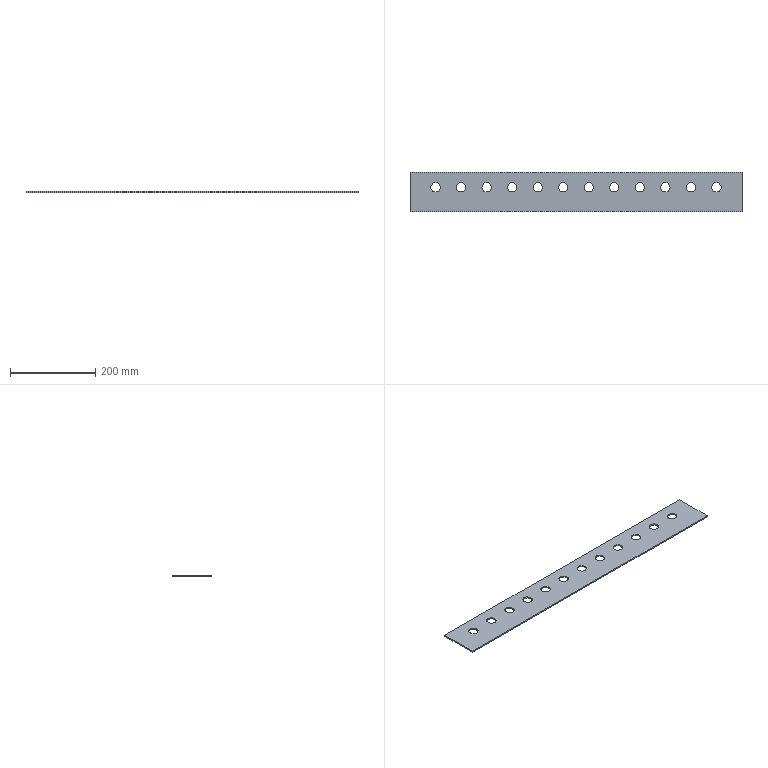Part | STEP file | Push button cover plate | 1 solid | 30 faces | box 780 x 92 x 3 mm | volume 201595 mm3 | cylinder 24 | plane 6 | commonest cylinder face diameters 22 x24